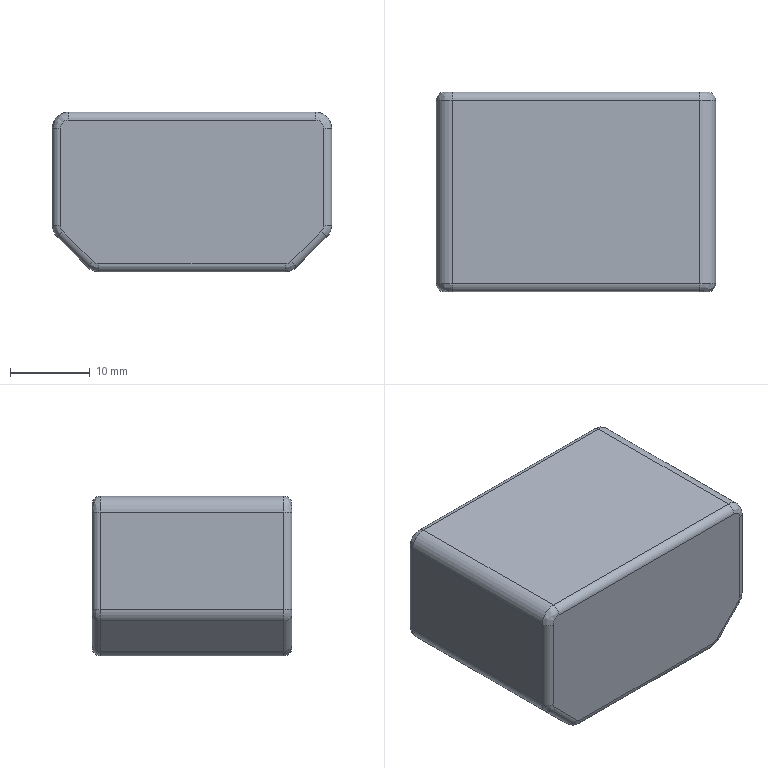Part | STEP file | 车灯-后视镜_id378_x_t | 1 solid | 38 faces | box 35 x 25 x 20 mm | volume 16780 mm3 | cylinder 18 | spline 12 | plane 8 | commonest cylinder face diameters 2 x12 4 x6
STEP:
#1=CARTESIAN_POINT('',(68.,-286.,-247.5));
#2=VERTEX_POINT('',#1);
#3=CARTESIAN_POINT('',(68.,-309.,-247.5));
#4=VERTEX_POINT('',#3);
#5=CARTESIAN_POINT('',(68.,-300.,-247.5));
#6=DIRECTION('',(0.,-1.,0.));
#7=VECTOR('',#6,1.);
#8=LINE('',#5,#7);
#9=EDGE_CURVE('',#2,#4,#8,.T.);
#10=ORIENTED_EDGE('',*,*,#9,.T.);
#11=CARTESIAN_POINT('',(99.,-309.,-247.5));
#12=VERTEX_POINT('',#11);
#13=CARTESIAN_POINT('',(83.5,-309.,-247.5));
#14=DIRECTION('',(1.,0.,0.));
#15=VECTOR('',#14,1.);
#16=LINE('',#13,#15);
#17=EDGE_CURVE('',#4,#12,#16,.T.);
#18=ORIENTED_EDGE('',*,*,#17,.T.);
#19=CARTESIAN_POINT('',(99.,-286.,-247.5));
#20=VERTEX_POINT('',#19);
#21=CARTESIAN_POINT('',(99.,-300.,-247.5));
#22=DIRECTION('',(0.,1.,0.));
#23=VECTOR('',#22,1.);
#24=LINE('',#21,#23);
#25=EDGE_CURVE('',#12,#20,#24,.T.);
#26=ORIENTED_EDGE('',*,*,#25,.T.);
#27=CARTESIAN_POINT('',(83.5,-286.,-247.5));
#28=DIRECTION('',(-1.,0.,0.));
#29=VECTOR('',#28,1.);
#30=LINE('',#27,#29);
#31=EDGE_CURVE('',#20,#2,#30,.T.);
#32=ORIENTED_EDGE('',*,*,#31,.T.);
#33=EDGE_LOOP('',(#10,#18,#26,#32));
#34=FACE_OUTER_BOUND('',#33,.T.);
#35=CARTESIAN_POINT('',(83.5,-300.,-247.5));
#36=DIRECTION('',(0.,0.,1.));
#37=DIRECTION('',(1.,0.,0.));
#38=AXIS2_PLACEMENT_3D('',#35,#36,#37);
#39=PLANE('',#38);
#40=ADVANCED_FACE('',(#34),#39,.T.);
#41=CARTESIAN_POINT('',(100.,-310.,-261.672));
#42=VERTEX_POINT('',#41);
#43=CARTESIAN_POINT('',(100.,-310.,-249.5));
#44=VERTEX_POINT('',#43);
#45=CARTESIAN_POINT('',(100.,-310.,-267.5));
#46=DIRECTION('',(0.,0.,1.));
#47=VECTOR('',#46,1.);
#48=LINE('',#45,#47);
#49=EDGE_CURVE('',#42,#44,#48,.T.);
#50=ORIENTED_EDGE('',*,*,#49,.T.);
#51=CARTESIAN_POINT('',(99.,-310.,-248.5));
#52=VERTEX_POINT('',#51);
#53=CARTESIAN_POINT('',(99.,-310.,-249.5));
#54=DIRECTION('',(0.,-1.,0.));
#55=DIRECTION('',(0.,0.,-1.));
#56=AXIS2_PLACEMENT_3D('',#53,#54,#55);
#57=CIRCLE('',#56,1.);
#58=EDGE_CURVE('',#44,#52,#57,.T.);
#59=ORIENTED_EDGE('',*,*,#58,.T.);
#60=CARTESIAN_POINT('',(68.,-310.,-248.5));
#61=VERTEX_POINT('',#60);
#62=CARTESIAN_POINT('',(83.5,-310.,-248.5));
#63=DIRECTION('',(-1.,0.,0.));
#64=VECTOR('',#63,1.);
#65=LINE('',#62,#64);
#66=EDGE_CURVE('',#52,#61,#65,.T.);
#67=ORIENTED_EDGE('',*,*,#66,.T.);
#68=CARTESIAN_POINT('',(67.,-310.,-249.5));
#69=VERTEX_POINT('',#68);
#70=CARTESIAN_POINT('',(68.,-310.,-249.5));
#71=DIRECTION('',(0.,-1.,0.));
#72=DIRECTION('',(0.,0.,-1.));
#73=AXIS2_PLACEMENT_3D('',#70,#71,#72);
#74=CIRCLE('',#73,1.);
#75=EDGE_CURVE('',#61,#69,#74,.T.);
#76=ORIENTED_EDGE('',*,*,#75,.T.);
#77=CARTESIAN_POINT('',(67.,-310.,-261.672));
#78=VERTEX_POINT('',#77);
#79=CARTESIAN_POINT('',(67.,-310.,-267.5));
#80=DIRECTION('',(0.,0.,-1.));
#81=VECTOR('',#80,1.);
#82=LINE('',#79,#81);
#83=EDGE_CURVE('',#69,#78,#82,.T.);
#84=ORIENTED_EDGE('',*,*,#83,.T.);
#85=CARTESIAN_POINT('',(67.293,-310.,-262.379));
#86=VERTEX_POINT('',#85);
#87=CARTESIAN_POINT('',(68.,-310.,-261.672));
#88=DIRECTION('',(0.,-1.,0.));
#89=DIRECTION('',(0.,0.,-1.));
#90=AXIS2_PLACEMENT_3D('',#87,#88,#89);
#91=CIRCLE('',#90,1.);
#92=EDGE_CURVE('',#78,#86,#91,.T.);
#93=ORIENTED_EDGE('',*,*,#92,.T.);
#94=CARTESIAN_POINT('',(71.121,-310.,-266.207));
#95=VERTEX_POINT('',#94);
#96=CARTESIAN_POINT('',(77.957,-310.,-273.043));
#97=DIRECTION('',(0.7071,0.,-0.7071));
#98=VECTOR('',#97,1.);
#99=LINE('',#96,#98);
#100=EDGE_CURVE('',#86,#95,#99,.T.);
#101=ORIENTED_EDGE('',*,*,#100,.T.);
#102=CARTESIAN_POINT('',(71.828,-310.,-266.5));
#103=VERTEX_POINT('',#102);
#104=CARTESIAN_POINT('',(71.828,-310.,-265.5));
#105=DIRECTION('',(0.,-1.,0.));
#106=DIRECTION('',(0.,0.,-1.));
#107=AXIS2_PLACEMENT_3D('',#104,#105,#106);
#108=CIRCLE('',#107,1.);
#109=EDGE_CURVE('',#95,#103,#108,.T.);
#110=ORIENTED_EDGE('',*,*,#109,.T.);
#111=CARTESIAN_POINT('',(95.172,-310.,-266.5));
#112=VERTEX_POINT('',#111);
#113=CARTESIAN_POINT('',(83.5,-310.,-266.5));
#114=DIRECTION('',(1.,0.,0.));
#115=VECTOR('',#114,1.);
#116=LINE('',#113,#115);
#117=EDGE_CURVE('',#103,#112,#116,.T.);
#118=ORIENTED_EDGE('',*,*,#117,.T.);
#119=CARTESIAN_POINT('',(95.879,-310.,-266.207));
#120=VERTEX_POINT('',#119);
#121=CARTESIAN_POINT('',(95.172,-310.,-265.5));
#122=DIRECTION('',(0.,-1.,0.));
#123=DIRECTION('',(0.,0.,-1.));
#124=AXIS2_PLACEMENT_3D('',#121,#122,#123);
#125=CIRCLE('',#124,1.);
#126=EDGE_CURVE('',#112,#120,#125,.T.);
#127=ORIENTED_EDGE('',*,*,#126,.T.);
#128=CARTESIAN_POINT('',(99.707,-310.,-262.379));
#129=VERTEX_POINT('',#128);
#130=CARTESIAN_POINT('',(89.043,-310.,-273.043));
#131=DIRECTION('',(0.7071,0.,0.7071));
#132=VECTOR('',#131,1.);
#133=LINE('',#130,#132);
#134=EDGE_CURVE('',#120,#129,#133,.T.);
#135=ORIENTED_EDGE('',*,*,#134,.T.);
#136=CARTESIAN_POINT('',(99.,-310.,-261.672));
#137=DIRECTION('',(0.,-1.,0.));
#138=DIRECTION('',(0.,0.,-1.));
#139=AXIS2_PLACEMENT_3D('',#136,#137,#138);
#140=CIRCLE('',#139,1.);
#141=EDGE_CURVE('',#129,#42,#140,.T.);
#142=ORIENTED_EDGE('',*,*,#141,.T.);
#143=EDGE_LOOP('',(#50,#59,#67,#76,#84,#93,#101,#110,#118,#127,#135,#142));
#144=FACE_OUTER_BOUND('',#143,.T.);
#145=CARTESIAN_POINT('',(83.5,-310.,-267.5));
#146=DIRECTION('',(0.,-1.,0.));
#147=DIRECTION('',(0.,0.,-1.));
#148=AXIS2_PLACEMENT_3D('',#145,#146,#147);
#149=PLANE('',#148);
#150=ADVANCED_FACE('',(#144),#149,.T.);
#151=CARTESIAN_POINT('',(66.,-286.,-261.672));
#152=VERTEX_POINT('',#151);
#153=CARTESIAN_POINT('',(66.,-309.,-261.672));
#154=VERTEX_POINT('',#153);
#155=CARTESIAN_POINT('',(66.,-300.,-261.672));
#156=DIRECTION('',(0.,-1.,0.));
#157=VECTOR('',#156,1.);
#158=LINE('',#155,#157);
#159=EDGE_CURVE('',#152,#154,#158,.T.);
#160=ORIENTED_EDGE('',*,*,#159,.T.);
#161=CARTESIAN_POINT('',(66.,-309.,-249.5));
#162=VERTEX_POINT('',#161);
#163=CARTESIAN_POINT('',(66.,-309.,-267.5));
#164=DIRECTION('',(0.,0.,1.));
#165=VECTOR('',#164,1.);
#166=LINE('',#163,#165);
#167=EDGE_CURVE('',#154,#162,#166,.T.);
#168=ORIENTED_EDGE('',*,*,#167,.T.);
#169=CARTESIAN_POINT('',(66.,-286.,-249.5));
#170=VERTEX_POINT('',#169);
#171=CARTESIAN_POINT('',(66.,-300.,-249.5));
#172=DIRECTION('',(0.,1.,0.));
#173=VECTOR('',#172,1.);
#174=LINE('',#171,#173);
#175=EDGE_CURVE('',#162,#170,#174,.T.);
#176=ORIENTED_EDGE('',*,*,#175,.T.);
#177=CARTESIAN_POINT('',(66.,-286.,-267.5));
#178=DIRECTION('',(0.,0.,-1.));
#179=VECTOR('',#178,1.);
#180=LINE('',#177,#179);
#181=EDGE_CURVE('',#170,#152,#180,.T.);
#182=ORIENTED_EDGE('',*,*,#181,.T.);
#183=EDGE_LOOP('',(#160,#168,#176,#182));
#184=FACE_OUTER_BOUND('',#183,.T.);
#185=CARTESIAN_POINT('',(66.,-300.,-267.5));
#186=DIRECTION('',(-1.,0.,0.));
#187=DIRECTION('',(0.,0.,1.));
#188=AXIS2_PLACEMENT_3D('',#185,#186,#187);
#189=PLANE('',#188);
#190=ADVANCED_FACE('',(#184),#189,.T.);
#191=CARTESIAN_POINT('',(67.,-285.,-261.672));
#192=VERTEX_POINT('',#191);
#193=CARTESIAN_POINT('',(67.,-285.,-249.5));
#194=VERTEX_POINT('',#193);
#195=CARTESIAN_POINT('',(67.,-285.,-267.5));
#196=DIRECTION('',(0.,0.,1.));
#197=VECTOR('',#196,1.);
#198=LINE('',#195,#197);
#199=EDGE_CURVE('',#192,#194,#198,.T.);
#200=ORIENTED_EDGE('',*,*,#199,.T.);
#201=CARTESIAN_POINT('',(68.,-285.,-248.5));
#202=VERTEX_POINT('',#201);
#203=CARTESIAN_POINT('',(68.,-285.,-249.5));
#204=DIRECTION('',(0.,1.,0.));
#205=DIRECTION('',(0.,0.,1.));
#206=AXIS2_PLACEMENT_3D('',#203,#204,#205);
#207=CIRCLE('',#206,1.);
#208=EDGE_CURVE('',#194,#202,#207,.T.);
#209=ORIENTED_EDGE('',*,*,#208,.T.);
#210=CARTESIAN_POINT('',(99.,-285.,-248.5));
#211=VERTEX_POINT('',#210);
#212=CARTESIAN_POINT('',(83.5,-285.,-248.5));
#213=DIRECTION('',(1.,0.,0.));
#214=VECTOR('',#213,1.);
#215=LINE('',#212,#214);
#216=EDGE_CURVE('',#202,#211,#215,.T.);
#217=ORIENTED_EDGE('',*,*,#216,.T.);
#218=CARTESIAN_POINT('',(100.,-285.,-249.5));
#219=VERTEX_POINT('',#218);
#220=CARTESIAN_POINT('',(99.,-285.,-249.5));
#221=DIRECTION('',(0.,1.,0.));
#222=DIRECTION('',(0.,0.,1.));
#223=AXIS2_PLACEMENT_3D('',#220,#221,#222);
#224=CIRCLE('',#223,1.);
#225=EDGE_CURVE('',#211,#219,#224,.T.);
#226=ORIENTED_EDGE('',*,*,#225,.T.);
#227=CARTESIAN_POINT('',(100.,-285.,-261.672));
#228=VERTEX_POINT('',#227);
#229=CARTESIAN_POINT('',(100.,-285.,-267.5));
#230=DIRECTION('',(0.,0.,-1.));
#231=VECTOR('',#230,1.);
#232=LINE('',#229,#231);
#233=EDGE_CURVE('',#219,#228,#232,.T.);
#234=ORIENTED_EDGE('',*,*,#233,.T.);
#235=CARTESIAN_POINT('',(99.707,-285.,-262.379));
#236=VERTEX_POINT('',#235);
#237=CARTESIAN_POINT('',(99.,-285.,-261.672));
#238=DIRECTION('',(0.,1.,0.));
#239=DIRECTION('',(0.,0.,1.));
#240=AXIS2_PLACEMENT_3D('',#237,#238,#239);
#241=CIRCLE('',#240,1.);
#242=EDGE_CURVE('',#228,#236,#241,.T.);
#243=ORIENTED_EDGE('',*,*,#242,.T.);
#244=CARTESIAN_POINT('',(95.879,-285.,-266.207));
#245=VERTEX_POINT('',#244);
#246=CARTESIAN_POINT('',(89.043,-285.,-273.043));
#247=DIRECTION('',(-0.7071,0.,-0.7071));
#248=VECTOR('',#247,1.);
#249=LINE('',#246,#248);
#250=EDGE_CURVE('',#236,#245,#249,.T.);
#251=ORIENTED_EDGE('',*,*,#250,.T.);
#252=CARTESIAN_POINT('',(95.172,-285.,-266.5));
#253=VERTEX_POINT('',#252);
#254=CARTESIAN_POINT('',(95.172,-285.,-265.5));
#255=DIRECTION('',(0.,1.,0.));
#256=DIRECTION('',(0.,0.,1.));
#257=AXIS2_PLACEMENT_3D('',#254,#255,#256);
#258=CIRCLE('',#257,1.);
#259=EDGE_CURVE('',#245,#253,#258,.T.);
#260=ORIENTED_EDGE('',*,*,#259,.T.);
#261=CARTESIAN_POINT('',(71.828,-285.,-266.5));
#262=VERTEX_POINT('',#261);
#263=CARTESIAN_POINT('',(83.5,-285.,-266.5));
#264=DIRECTION('',(-1.,0.,0.));
#265=VECTOR('',#264,1.);
#266=LINE('',#263,#265);
#267=EDGE_CURVE('',#253,#262,#266,.T.);
#268=ORIENTED_EDGE('',*,*,#267,.T.);
#269=CARTESIAN_POINT('',(71.121,-285.,-266.207));
#270=VERTEX_POINT('',#269);
#271=CARTESIAN_POINT('',(71.828,-285.,-265.5));
#272=DIRECTION('',(0.,1.,0.));
#273=DIRECTION('',(0.,0.,1.));
#274=AXIS2_PLACEMENT_3D('',#271,#272,#273);
#275=CIRCLE('',#274,1.);
#276=EDGE_CURVE('',#262,#270,#275,.T.);
#277=ORIENTED_EDGE('',*,*,#276,.T.);
#278=CARTESIAN_POINT('',(67.293,-285.,-262.379));
#279=VERTEX_POINT('',#278);
#280=CARTESIAN_POINT('',(77.957,-285.,-273.043));
#281=DIRECTION('',(-0.7071,0.,0.7071));
#282=VECTOR('',#281,1.);
#283=LINE('',#280,#282);
#284=EDGE_CURVE('',#270,#279,#283,.T.);
#285=ORIENTED_EDGE('',*,*,#284,.T.);
#286=CARTESIAN_POINT('',(68.,-285.,-261.672));
#287=DIRECTION('',(0.,1.,0.));
#288=DIRECTION('',(0.,0.,1.));
#289=AXIS2_PLACEMENT_3D('',#286,#287,#288);
#290=CIRCLE('',#289,1.);
#291=EDGE_CURVE('',#279,#192,#290,.T.);
#292=ORIENTED_EDGE('',*,*,#291,.T.);
#293=EDGE_LOOP('',(#200,#209,#217,#226,#234,#243,#251,#260,#268,#277,#285,#292));
#294=FACE_OUTER_BOUND('',#293,.T.);
#295=CARTESIAN_POINT('',(83.5,-285.,-267.5));
#296=DIRECTION('',(0.,1.,0.));
#297=DIRECTION('',(0.,0.,1.));
#298=AXIS2_PLACEMENT_3D('',#295,#296,#297);
#299=PLANE('',#298);
#300=ADVANCED_FACE('',(#294),#299,.T.);
#301=CARTESIAN_POINT('',(95.172,-286.,-267.5));
#302=VERTEX_POINT('',#301);
#303=CARTESIAN_POINT('',(95.172,-309.,-267.5));
#304=VERTEX_POINT('',#303);
#305=CARTESIAN_POINT('',(95.172,-300.,-267.5));
#306=DIRECTION('',(0.,-1.,0.));
#307=VECTOR('',#306,1.);
#308=LINE('',#305,#307);
#309=EDGE_CURVE('',#302,#304,#308,.T.);
#310=ORIENTED_EDGE('',*,*,#309,.T.);
#311=CARTESIAN_POINT('',(71.828,-309.,-267.5));
#312=VERTEX_POINT('',#311);
#313=CARTESIAN_POINT('',(83.5,-309.,-267.5));
#314=DIRECTION('',(-1.,0.,0.));
#315=VECTOR('',#314,1.);
#316=LINE('',#313,#315);
#317=EDGE_CURVE('',#304,#312,#316,.T.);
#318=ORIENTED_EDGE('',*,*,#317,.T.);
#319=CARTESIAN_POINT('',(71.828,-286.,-267.5));
#320=VERTEX_POINT('',#319);
#321=CARTESIAN_POINT('',(71.828,-300.,-267.5));
#322=DIRECTION('',(0.,1.,0.));
#323=VECTOR('',#322,1.);
#324=LINE('',#321,#323);
#325=EDGE_CURVE('',#312,#320,#324,.T.);
#326=ORIENTED_EDGE('',*,*,#325,.T.);
#327=CARTESIAN_POINT('',(83.5,-286.,-267.5));
#328=DIRECTION('',(1.,0.,0.));
#329=VECTOR('',#328,1.);
#330=LINE('',#327,#329);
#331=EDGE_CURVE('',#320,#302,#330,.T.);
#332=ORIENTED_EDGE('',*,*,#331,.T.);
#333=EDGE_LOOP('',(#310,#318,#326,#332));
#334=FACE_OUTER_BOUND('',#333,.T.);
#335=CARTESIAN_POINT('',(83.5,-300.,-267.5));
#336=DIRECTION('',(0.,0.,-1.));
#337=DIRECTION('',(-1.,0.,0.));
#338=AXIS2_PLACEMENT_3D('',#335,#336,#337);
#339=PLANE('',#338);
#340=ADVANCED_FACE('',(#334),#339,.T.);
#341=CARTESIAN_POINT('',(101.,-286.,-249.5));
#342=VERTEX_POINT('',#341);
#343=CARTESIAN_POINT('',(101.,-309.,-249.5));
#344=VERTEX_POINT('',#343);
#345=CARTESIAN_POINT('',(101.,-300.,-249.5));
#346=DIRECTION('',(0.,-1.,0.));
#347=VECTOR('',#346,1.);
#348=LINE('',#345,#347);
#349=EDGE_CURVE('',#342,#344,#348,.T.);
#350=ORIENTED_EDGE('',*,*,#349,.T.);
#351=CARTESIAN_POINT('',(101.,-309.,-261.672));
#352=VERTEX_POINT('',#351);
#353=CARTESIAN_POINT('',(101.,-309.,-267.5));
#354=DIRECTION('',(0.,0.,-1.));
#355=VECTOR('',#354,1.);
#356=LINE('',#353,#355);
#357=EDGE_CURVE('',#344,#352,#356,.T.);
#358=ORIENTED_EDGE('',*,*,#357,.T.);
#359=CARTESIAN_POINT('',(101.,-286.,-261.672));
#360=VERTEX_POINT('',#359);
#361=CARTESIAN_POINT('',(101.,-300.,-261.672));
#362=DIRECTION('',(0.,1.,0.));
#363=VECTOR('',#362,1.);
#364=LINE('',#361,#363);
#365=EDGE_CURVE('',#352,#360,#364,.T.);
#366=ORIENTED_EDGE('',*,*,#365,.T.);
#367=CARTESIAN_POINT('',(101.,-286.,-267.5));
#368=DIRECTION('',(0.,0.,1.));
#369=VECTOR('',#368,1.);
#370=LINE('',#367,#369);
#371=EDGE_CURVE('',#360,#342,#370,.T.);
#372=ORIENTED_EDGE('',*,*,#371,.T.);
#373=EDGE_LOOP('',(#350,#358,#366,#372));
#374=FACE_OUTER_BOUND('',#373,.T.);
#375=CARTESIAN_POINT('',(101.,-300.,-267.5));
#376=DIRECTION('',(1.,0.,0.));
#377=DIRECTION('',(0.,0.,-1.));
#378=AXIS2_PLACEMENT_3D('',#375,#376,#377);
#379=PLANE('',#378);
#380=ADVANCED_FACE('',(#374),#379,.T.);
#381=CARTESIAN_POINT('',(70.414,-286.,-266.914));
#382=VERTEX_POINT('',#381);
#383=CARTESIAN_POINT('',(70.414,-309.,-266.914));
#384=VERTEX_POINT('',#383);
#385=CARTESIAN_POINT('',(70.414,-300.,-266.914));
#386=DIRECTION('',(0.,-1.,0.));
#387=VECTOR('',#386,1.);
#388=LINE('',#385,#387);
#389=EDGE_CURVE('',#382,#384,#388,.T.);
#390=ORIENTED_EDGE('',*,*,#389,.T.);
#391=CARTESIAN_POINT('',(66.586,-309.,-263.086));
#392=VERTEX_POINT('',#391);
#393=CARTESIAN_POINT('',(66.,-309.,-262.5));
#394=DIRECTION('',(-0.7071,0.,0.7071));
#395=VECTOR('',#394,1.);
#396=LINE('',#393,#395);
#397=EDGE_CURVE('',#384,#392,#396,.T.);
#398=ORIENTED_EDGE('',*,*,#397,.T.);
#399=CARTESIAN_POINT('',(66.586,-286.,-263.086));
#400=VERTEX_POINT('',#399);
#401=CARTESIAN_POINT('',(66.586,-300.,-263.086));
#402=DIRECTION('',(0.,1.,0.));
#403=VECTOR('',#402,1.);
#404=LINE('',#401,#403);
#405=EDGE_CURVE('',#392,#400,#404,.T.);
#406=ORIENTED_EDGE('',*,*,#405,.T.);
#407=CARTESIAN_POINT('',(66.,-286.,-262.5));
#408=DIRECTION('',(0.7071,0.,-0.7071));
#409=VECTOR('',#408,1.);
#410=LINE('',#407,#409);
#411=EDGE_CURVE('',#400,#382,#410,.T.);
#412=ORIENTED_EDGE('',*,*,#411,.T.);
#413=EDGE_LOOP('',(#390,#398,#406,#412));
#414=FACE_OUTER_BOUND('',#413,.T.);
#415=CARTESIAN_POINT('',(66.,-300.,-262.5));
#416=DIRECTION('',(0.7071,0.,0.7071));
#417=DIRECTION('',(0.7071,0.,-0.7071));
#418=AXIS2_PLACEMENT_3D('',#415,#416,#417);
#419=PLANE('',#418);
#420=ADVANCED_FACE('',(#414),#419,.F.);
#421=CARTESIAN_POINT('',(100.414,-286.,-263.086));
#422=VERTEX_POINT('',#421);
#423=CARTESIAN_POINT('',(100.414,-309.,-263.086));
#424=VERTEX_POINT('',#423);
#425=CARTESIAN_POINT('',(100.414,-300.,-263.086));
#426=DIRECTION('',(0.,-1.,0.));
#427=VECTOR('',#426,1.);
#428=LINE('',#425,#427);
#429=EDGE_CURVE('',#422,#424,#428,.T.);
#430=ORIENTED_EDGE('',*,*,#429,.T.);
#431=CARTESIAN_POINT('',(96.586,-309.,-266.914));
#432=VERTEX_POINT('',#431);
#433=CARTESIAN_POINT('',(101.,-309.,-262.5));
#434=DIRECTION('',(-0.7071,0.,-0.7071));
#435=VECTOR('',#434,1.);
#436=LINE('',#433,#435);
#437=EDGE_CURVE('',#424,#432,#436,.T.);
#438=ORIENTED_EDGE('',*,*,#437,.T.);
#439=CARTESIAN_POINT('',(96.586,-286.,-266.914));
#440=VERTEX_POINT('',#439);
#441=CARTESIAN_POINT('',(96.586,-300.,-266.914));
#442=DIRECTION('',(0.,1.,0.));
#443=VECTOR('',#442,1.);
#444=LINE('',#441,#443);
#445=EDGE_CURVE('',#432,#440,#444,.T.);
#446=ORIENTED_EDGE('',*,*,#445,.T.);
#447=CARTESIAN_POINT('',(101.,-286.,-262.5));
#448=DIRECTION('',(0.7071,0.,0.7071));
#449=VECTOR('',#448,1.);
#450=LINE('',#447,#449);
#451=EDGE_CURVE('',#440,#422,#450,.T.);
#452=ORIENTED_EDGE('',*,*,#451,.T.);
#453=EDGE_LOOP('',(#430,#438,#446,#452));
#454=FACE_OUTER_BOUND('',#453,.T.);
#455=CARTESIAN_POINT('',(101.,-300.,-262.5));
#456=DIRECTION('',(-0.7071,0.,0.7071));
#457=DIRECTION('',(0.7071,0.,0.7071));
#458=AXIS2_PLACEMENT_3D('',#455,#456,#457);
#459=PLANE('',#458);
#460=ADVANCED_FACE('',(#454),#459,.F.);
#461=ORIENTED_EDGE('',*,*,#445,.F.);
#462=CARTESIAN_POINT('',(95.172,-309.,-265.5));
#463=DIRECTION('',(0.,1.,0.));
#464=DIRECTION('',(0.,0.,-1.));
#465=AXIS2_PLACEMENT_3D('',#462,#463,#464);
#466=CIRCLE('',#465,2.);
#467=EDGE_CURVE('',#432,#304,#466,.T.);
#468=ORIENTED_EDGE('',*,*,#467,.T.);
#469=ORIENTED_EDGE('',*,*,#309,.F.);
#470=CARTESIAN_POINT('',(95.172,-286.,-265.5));
#471=DIRECTION('',(0.,-1.,0.));
#472=DIRECTION('',(0.,0.,1.));
#473=AXIS2_PLACEMENT_3D('',#470,#471,#472);
#474=CIRCLE('',#473,2.);
#475=EDGE_CURVE('',#302,#440,#474,.T.);
#476=ORIENTED_EDGE('',*,*,#475,.T.);
#477=EDGE_LOOP('',(#461,#468,#469,#476));
#478=FACE_OUTER_BOUND('',#477,.T.);
#479=CARTESIAN_POINT('',(95.172,-300.,-265.5));
#480=DIRECTION('',(0.,1.,0.));
#481=DIRECTION('',(0.,0.,1.));
#482=AXIS2_PLACEMENT_3D('',#479,#480,#481);
#483=CYLINDRICAL_SURFACE('',#482,2.);
#484=ADVANCED_FACE('',(#478),#483,.T.);
#485=ORIENTED_EDGE('',*,*,#365,.F.);
#486=CARTESIAN_POINT('',(99.,-309.,-261.672));
#487=DIRECTION('',(0.,1.,0.));
#488=DIRECTION('',(0.,0.,-1.));
#489=AXIS2_PLACEMENT_3D('',#486,#487,#488);
#490=CIRCLE('',#489,2.);
#491=EDGE_CURVE('',#352,#424,#490,.T.);
#492=ORIENTED_EDGE('',*,*,#491,.T.);
#493=ORIENTED_EDGE('',*,*,#429,.F.);
#494=CARTESIAN_POINT('',(99.,-286.,-261.672));
#495=DIRECTION('',(0.,-1.,0.));
#496=DIRECTION('',(0.,0.,1.));
#497=AXIS2_PLACEMENT_3D('',#494,#495,#496);
#498=CIRCLE('',#497,2.);
#499=EDGE_CURVE('',#422,#360,#498,.T.);
#500=ORIENTED_EDGE('',*,*,#499,.T.);
#501=EDGE_LOOP('',(#485,#492,#493,#500));
#502=FACE_OUTER_BOUND('',#501,.T.);
#503=CARTESIAN_POINT('',(99.,-300.,-261.672));
#504=DIRECTION('',(0.,-1.,0.));
#505=DIRECTION('',(0.,0.,-1.));
#506=AXIS2_PLACEMENT_3D('',#503,#504,#505);
#507=CYLINDRICAL_SURFACE('',#506,2.);
#508=ADVANCED_FACE('',(#502),#507,.T.);
#509=ORIENTED_EDGE('',*,*,#25,.F.);
#510=CARTESIAN_POINT('',(99.,-309.,-249.5));
#511=DIRECTION('',(0.,1.,0.));
#512=DIRECTION('',(0.,0.,-1.));
#513=AXIS2_PLACEMENT_3D('',#510,#511,#512);
#514=CIRCLE('',#513,2.);
#515=EDGE_CURVE('',#12,#344,#514,.T.);
#516=ORIENTED_EDGE('',*,*,#515,.T.);
#517=ORIENTED_EDGE('',*,*,#349,.F.);
#518=CARTESIAN_POINT('',(99.,-286.,-249.5));
#519=DIRECTION('',(0.,-1.,0.));
#520=DIRECTION('',(0.,0.,1.));
#521=AXIS2_PLACEMENT_3D('',#518,#519,#520);
#522=CIRCLE('',#521,2.);
#523=EDGE_CURVE('',#342,#20,#522,.T.);
#524=ORIENTED_EDGE('',*,*,#523,.T.);
#525=EDGE_LOOP('',(#509,#516,#517,#524));
#526=FACE_OUTER_BOUND('',#525,.T.);
#527=CARTESIAN_POINT('',(99.,-300.,-249.5));
#528=DIRECTION('',(0.,-1.,0.));
#529=DIRECTION('',(0.,0.,-1.));
#530=AXIS2_PLACEMENT_3D('',#527,#528,#529);
#531=CYLINDRICAL_SURFACE('',#530,2.);
#532=ADVANCED_FACE('',(#526),#531,.T.);
#533=ORIENTED_EDGE('',*,*,#175,.F.);
#534=CARTESIAN_POINT('',(68.,-309.,-249.5));
#535=DIRECTION('',(0.,1.,0.));
#536=DIRECTION('',(0.,0.,-1.));
#537=AXIS2_PLACEMENT_3D('',#534,#535,#536);
#538=CIRCLE('',#537,2.);
#539=EDGE_CURVE('',#162,#4,#538,.T.);
#540=ORIENTED_EDGE('',*,*,#539,.T.);
#541=ORIENTED_EDGE('',*,*,#9,.F.);
#542=CARTESIAN_POINT('',(68.,-286.,-249.5));
#543=DIRECTION('',(0.,-1.,0.));
#544=DIRECTION('',(0.,0.,1.));
#545=AXIS2_PLACEMENT_3D('',#542,#543,#544);
#546=CIRCLE('',#545,2.);
#547=EDGE_CURVE('',#2,#170,#546,.T.);
#548=ORIENTED_EDGE('',*,*,#547,.T.);
#549=EDGE_LOOP('',(#533,#540,#541,#548));
#550=FACE_OUTER_BOUND('',#549,.T.);
#551=CARTESIAN_POINT('',(68.,-300.,-249.5));
#552=DIRECTION('',(0.,1.,0.));
#553=DIRECTION('',(0.,0.,1.));
#554=AXIS2_PLACEMENT_3D('',#551,#552,#553);
#555=CYLINDRICAL_SURFACE('',#554,2.);
#556=ADVANCED_FACE('',(#550),#555,.T.);
#557=ORIENTED_EDGE('',*,*,#325,.F.);
#558=CARTESIAN_POINT('',(71.828,-309.,-265.5));
#559=DIRECTION('',(0.,1.,0.));
#560=DIRECTION('',(0.,0.,-1.));
#561=AXIS2_PLACEMENT_3D('',#558,#559,#560);
#562=CIRCLE('',#561,2.);
#563=EDGE_CURVE('',#312,#384,#562,.T.);
#564=ORIENTED_EDGE('',*,*,#563,.T.);
#565=ORIENTED_EDGE('',*,*,#389,.F.);
#566=CARTESIAN_POINT('',(71.828,-286.,-265.5));
#567=DIRECTION('',(0.,-1.,0.));
#568=DIRECTION('',(0.,0.,1.));
#569=AXIS2_PLACEMENT_3D('',#566,#567,#568);
#570=CIRCLE('',#569,2.);
#571=EDGE_CURVE('',#382,#320,#570,.T.);
#572=ORIENTED_EDGE('',*,*,#571,.T.);
#573=EDGE_LOOP('',(#557,#564,#565,#572));
#574=FACE_OUTER_BOUND('',#573,.T.);
#575=CARTESIAN_POINT('',(71.828,-300.,-265.5));
#576=DIRECTION('',(0.,-1.,0.));
#577=DIRECTION('',(0.,0.,-1.));
#578=AXIS2_PLACEMENT_3D('',#575,#576,#577);
#579=CYLINDRICAL_SURFACE('',#578,2.);
#580=ADVANCED_FACE('',(#574),#579,.T.);
#581=ORIENTED_EDGE('',*,*,#405,.F.);
#582=CARTESIAN_POINT('',(68.,-309.,-261.672));
#583=DIRECTION('',(0.,1.,0.));
#584=DIRECTION('',(0.,0.,-1.));
#585=AXIS2_PLACEMENT_3D('',#582,#583,#584);
#586=CIRCLE('',#585,2.);
#587=EDGE_CURVE('',#392,#154,#586,.T.);
#588=ORIENTED_EDGE('',*,*,#587,.T.);
#589=ORIENTED_EDGE('',*,*,#159,.F.);
#590=CARTESIAN_POINT('',(68.,-286.,-261.672));
#591=DIRECTION('',(0.,-1.,0.));
#592=DIRECTION('',(0.,0.,1.));
#593=AXIS2_PLACEMENT_3D('',#590,#591,#592);
#594=CIRCLE('',#593,2.);
#595=EDGE_CURVE('',#152,#400,#594,.T.);
#596=ORIENTED_EDGE('',*,*,#595,.T.);
#597=EDGE_LOOP('',(#581,#588,#589,#596));
#598=FACE_OUTER_BOUND('',#597,.T.);
#599=CARTESIAN_POINT('',(68.,-300.,-261.672));
#600=DIRECTION('',(0.,1.,0.));
#601=DIRECTION('',(0.,0.,1.));
#602=AXIS2_PLACEMENT_3D('',#599,#600,#601);
#603=CYLINDRICAL_SURFACE('',#602,2.);
#604=ADVANCED_FACE('',(#598),#603,.T.);
#605=CARTESIAN_POINT('',(71.121,-309.,-266.207));
#606=DIRECTION('',(-0.7071,0.,0.7071));
#607=DIRECTION('',(0.7071,0.,0.7071));
#608=AXIS2_PLACEMENT_3D('',#605,#606,#607);
#609=CIRCLE('',#608,1.);
#610=EDGE_CURVE('',#384,#95,#609,.T.);
#611=ORIENTED_EDGE('',*,*,#610,.F.);
#612=ORIENTED_EDGE('',*,*,#563,.F.);
#613=CARTESIAN_POINT('',(71.828,-309.,-266.5));
#614=DIRECTION('',(1.,0.,0.));
#615=DIRECTION('',(0.,0.,-1.));
#616=AXIS2_PLACEMENT_3D('',#613,#614,#615);
#617=CIRCLE('',#616,1.);
#618=EDGE_CURVE('',#103,#312,#617,.T.);
#619=ORIENTED_EDGE('',*,*,#618,.F.);
#620=ORIENTED_EDGE('',*,*,#109,.F.);
#621=EDGE_LOOP('',(#611,#612,#619,#620));
#622=FACE_OUTER_BOUND('',#621,.T.);
#623=CARTESIAN_POINT('',(71.121,-310.,-266.207));
#624=CARTESIAN_POINT('',(71.311,-310.,-266.397));
#625=CARTESIAN_POINT('',(71.56,-310.,-266.5));
#626=CARTESIAN_POINT('',(71.828,-310.,-266.5));
#627=CARTESIAN_POINT('',(70.707,-310.,-266.621));
#628=CARTESIAN_POINT('',(71.008,-310.,-266.923));
#629=CARTESIAN_POINT('',(71.402,-310.,-267.086));
#630=CARTESIAN_POINT('',(71.828,-310.,-267.086));
#631=CARTESIAN_POINT('',(70.414,-309.586,-266.914));
#632=CARTESIAN_POINT('',(70.794,-309.586,-267.294));
#633=CARTESIAN_POINT('',(71.291,-309.586,-267.5));
#634=CARTESIAN_POINT('',(71.828,-309.586,-267.5));
#635=CARTESIAN_POINT('',(70.414,-309.,-266.914));
#636=CARTESIAN_POINT('',(70.794,-309.,-267.294));
#637=CARTESIAN_POINT('',(71.291,-309.,-267.5));
#638=CARTESIAN_POINT('',(71.828,-309.,-267.5));
#639=(BOUNDED_SURFACE()B_SPLINE_SURFACE(3,3,((#623,#624,#625,#626),(#627,#628,#629,#630),(#631,#632,#633,#634),(#635,#636,#637,#638)),.UNSPECIFIED.,.F.,.F.,.F.)B_SPLINE_SURFACE_WITH_KNOTS((4,4),(4,4),(0.,1.),(0.,1.),.UNSPECIFIED.)GEOMETRIC_REPRESENTATION_ITEM()RATIONAL_B_SPLINE_SURFACE(((1.,0.9493,0.9493,1.),(0.8047,0.7639,0.7639,0.8047),(0.8047,0.7639,0.7639,0.8047),(1.,0.9493,0.9493,1.)))REPRESENTATION_ITEM('')SURFACE());
#640=ADVANCED_FACE('',(#622),#639,.T.);
#641=ORIENTED_EDGE('',*,*,#618,.T.);
#642=ORIENTED_EDGE('',*,*,#317,.F.);
#643=CARTESIAN_POINT('',(95.172,-309.,-266.5));
#644=DIRECTION('',(1.,0.,0.));
#645=DIRECTION('',(0.,0.,-1.));
#646=AXIS2_PLACEMENT_3D('',#643,#644,#645);
#647=CIRCLE('',#646,1.);
#648=EDGE_CURVE('',#112,#304,#647,.T.);
#649=ORIENTED_EDGE('',*,*,#648,.F.);
#650=ORIENTED_EDGE('',*,*,#117,.F.);
#651=EDGE_LOOP('',(#641,#642,#649,#650));
#652=FACE_OUTER_BOUND('',#651,.T.);
#653=CARTESIAN_POINT('',(83.5,-309.,-266.5));
#654=DIRECTION('',(1.,0.,0.));
#655=DIRECTION('',(0.,0.,-1.));
#656=AXIS2_PLACEMENT_3D('',#653,#654,#655);
#657=CYLINDRICAL_SURFACE('',#656,1.);
#658=ADVANCED_FACE('',(#652),#657,.T.);
#659=ORIENTED_EDGE('',*,*,#610,.T.);
#660=ORIENTED_EDGE('',*,*,#100,.F.);
#661=CARTESIAN_POINT('',(67.293,-309.,-262.379));
#662=DIRECTION('',(-0.7071,0.,0.7071));
#663=DIRECTION('',(0.7071,0.,0.7071));
#664=AXIS2_PLACEMENT_3D('',#661,#662,#663);
#665=CIRCLE('',#664,1.);
#666=EDGE_CURVE('',#392,#86,#665,.T.);
#667=ORIENTED_EDGE('',*,*,#666,.F.);
#668=ORIENTED_EDGE('',*,*,#397,.F.);
#669=EDGE_LOOP('',(#659,#660,#667,#668));
#670=FACE_OUTER_BOUND('',#669,.T.);
#671=CARTESIAN_POINT('',(77.957,-309.,-273.043));
#672=DIRECTION('',(-0.7071,0.,0.7071));
#673=DIRECTION('',(0.7071,0.,0.7071));
#674=AXIS2_PLACEMENT_3D('',#671,#672,#673);
#675=CYLINDRICAL_SURFACE('',#674,1.);
#676=ADVANCED_FACE('',(#670),#675,.T.);
#677=ORIENTED_EDGE('',*,*,#648,.T.);
#678=ORIENTED_EDGE('',*,*,#467,.F.);
#679=CARTESIAN_POINT('',(95.879,-309.,-266.207));
#680=DIRECTION('',(0.7071,0.,0.7071));
#681=DIRECTION('',(0.7071,0.,-0.7071));
#682=AXIS2_PLACEMENT_3D('',#679,#680,#681);
#683=CIRCLE('',#682,1.);
#684=EDGE_CURVE('',#120,#432,#683,.T.);
#685=ORIENTED_EDGE('',*,*,#684,.F.);
#686=ORIENTED_EDGE('',*,*,#126,.F.);
#687=EDGE_LOOP('',(#677,#678,#685,#686));
#688=FACE_OUTER_BOUND('',#687,.T.);
#689=CARTESIAN_POINT('',(95.172,-310.,-266.5));
#690=CARTESIAN_POINT('',(95.44,-310.,-266.5));
#691=CARTESIAN_POINT('',(95.689,-310.,-266.397));
#692=CARTESIAN_POINT('',(95.879,-310.,-266.207));
#693=CARTESIAN_POINT('',(95.172,-310.,-267.086));
#694=CARTESIAN_POINT('',(95.598,-310.,-267.086));
#695=CARTESIAN_POINT('',(95.992,-310.,-266.923));
#696=CARTESIAN_POINT('',(96.293,-310.,-266.621));
#697=CARTESIAN_POINT('',(95.172,-309.586,-267.5));
#698=CARTESIAN_POINT('',(95.709,-309.586,-267.5));
#699=CARTESIAN_POINT('',(96.206,-309.586,-267.294));
#700=CARTESIAN_POINT('',(96.586,-309.586,-266.914));
#701=CARTESIAN_POINT('',(95.172,-309.,-267.5));
#702=CARTESIAN_POINT('',(95.709,-309.,-267.5));
#703=CARTESIAN_POINT('',(96.206,-309.,-267.294));
#704=CARTESIAN_POINT('',(96.586,-309.,-266.914));
#705=(BOUNDED_SURFACE()B_SPLINE_SURFACE(3,3,((#689,#690,#691,#692),(#693,#694,#695,#696),(#697,#698,#699,#700),(#701,#702,#703,#704)),.UNSPECIFIED.,.F.,.F.,.F.)B_SPLINE_SURFACE_WITH_KNOTS((4,4),(4,4),(0.,1.),(0.,1.),.UNSPECIFIED.)GEOMETRIC_REPRESENTATION_ITEM()RATIONAL_B_SPLINE_SURFACE(((1.,0.9493,0.9493,1.),(0.8047,0.7639,0.7639,0.8047),(0.8047,0.7639,0.7639,0.8047),(1.,0.9493,0.9493,1.)))REPRESENTATION_ITEM('')SURFACE());
#706=ADVANCED_FACE('',(#688),#705,.T.);
#707=ORIENTED_EDGE('',*,*,#666,.T.);
#708=ORIENTED_EDGE('',*,*,#92,.F.);
#709=CARTESIAN_POINT('',(67.,-309.,-261.672));
#710=DIRECTION('',(0.,0.,1.));
#711=DIRECTION('',(1.,0.,0.));
#712=AXIS2_PLACEMENT_3D('',#709,#710,#711);
#713=CIRCLE('',#712,1.);
#714=EDGE_CURVE('',#154,#78,#713,.T.);
#715=ORIENTED_EDGE('',*,*,#714,.F.);
#716=ORIENTED_EDGE('',*,*,#587,.F.);
#717=EDGE_LOOP('',(#707,#708,#715,#716));
#718=FACE_OUTER_BOUND('',#717,.T.);
#719=CARTESIAN_POINT('',(67.,-310.,-261.672));
#720=CARTESIAN_POINT('',(67.,-310.,-261.94));
#721=CARTESIAN_POINT('',(67.103,-310.,-262.189));
#722=CARTESIAN_POINT('',(67.293,-310.,-262.379));
#723=CARTESIAN_POINT('',(66.414,-310.,-261.672));
#724=CARTESIAN_POINT('',(66.414,-310.,-262.098));
#725=CARTESIAN_POINT('',(66.577,-310.,-262.492));
#726=CARTESIAN_POINT('',(66.879,-310.,-262.793));
#727=CARTESIAN_POINT('',(66.,-309.586,-261.672));
#728=CARTESIAN_POINT('',(66.,-309.586,-262.209));
#729=CARTESIAN_POINT('',(66.206,-309.586,-262.706));
#730=CARTESIAN_POINT('',(66.586,-309.586,-263.086));
#731=CARTESIAN_POINT('',(66.,-309.,-261.672));
#732=CARTESIAN_POINT('',(66.,-309.,-262.209));
#733=CARTESIAN_POINT('',(66.206,-309.,-262.706));
#734=CARTESIAN_POINT('',(66.586,-309.,-263.086));
#735=(BOUNDED_SURFACE()B_SPLINE_SURFACE(3,3,((#719,#720,#721,#722),(#723,#724,#725,#726),(#727,#728,#729,#730),(#731,#732,#733,#734)),.UNSPECIFIED.,.F.,.F.,.F.)B_SPLINE_SURFACE_WITH_KNOTS((4,4),(4,4),(0.,1.),(0.,1.),.UNSPECIFIED.)GEOMETRIC_REPRESENTATION_ITEM()RATIONAL_B_SPLINE_SURFACE(((1.,0.9493,0.9493,1.),(0.8047,0.7639,0.7639,0.8047),(0.8047,0.7639,0.7639,0.8047),(1.,0.9493,0.9493,1.)))REPRESENTATION_ITEM('')SURFACE());
#736=ADVANCED_FACE('',(#718),#735,.T.);
#737=ORIENTED_EDGE('',*,*,#684,.T.);
#738=ORIENTED_EDGE('',*,*,#437,.F.);
#739=CARTESIAN_POINT('',(99.707,-309.,-262.379));
#740=DIRECTION('',(0.7071,0.,0.7071));
#741=DIRECTION('',(0.7071,0.,-0.7071));
#742=AXIS2_PLACEMENT_3D('',#739,#740,#741);
#743=CIRCLE('',#742,1.);
#744=EDGE_CURVE('',#129,#424,#743,.T.);
#745=ORIENTED_EDGE('',*,*,#744,.F.);
#746=ORIENTED_EDGE('',*,*,#134,.F.);
#747=EDGE_LOOP('',(#737,#738,#745,#746));
#748=FACE_OUTER_BOUND('',#747,.T.);
#749=CARTESIAN_POINT('',(89.043,-309.,-273.043));
#750=DIRECTION('',(-0.7071,0.,-0.7071));
#751=DIRECTION('',(-0.7071,0.,0.7071));
#752=AXIS2_PLACEMENT_3D('',#749,#750,#751);
#753=CYLINDRICAL_SURFACE('',#752,1.);
#754=ADVANCED_FACE('',(#748),#753,.T.);
#755=ORIENTED_EDGE('',*,*,#714,.T.);
#756=ORIENTED_EDGE('',*,*,#83,.F.);
#757=CARTESIAN_POINT('',(67.,-309.,-249.5));
#758=DIRECTION('',(0.,0.,1.));
#759=DIRECTION('',(1.,0.,0.));
#760=AXIS2_PLACEMENT_3D('',#757,#758,#759);
#761=CIRCLE('',#760,1.);
#762=EDGE_CURVE('',#162,#69,#761,.T.);
#763=ORIENTED_EDGE('',*,*,#762,.F.);
#764=ORIENTED_EDGE('',*,*,#167,.F.);
#765=EDGE_LOOP('',(#755,#756,#763,#764));
#766=FACE_OUTER_BOUND('',#765,.T.);
#767=CARTESIAN_POINT('',(67.,-309.,-267.5));
#768=DIRECTION('',(0.,0.,1.));
#769=DIRECTION('',(1.,0.,0.));
#770=AXIS2_PLACEMENT_3D('',#767,#768,#769);
#771=CYLINDRICAL_SURFACE('',#770,1.);
#772=ADVANCED_FACE('',(#766),#771,.T.);
#773=ORIENTED_EDGE('',*,*,#744,.T.);
#774=ORIENTED_EDGE('',*,*,#491,.F.);
#775=CARTESIAN_POINT('',(100.,-309.,-261.672));
#776=DIRECTION('',(0.,0.,1.));
#777=DIRECTION('',(1.,0.,0.));
#778=AXIS2_PLACEMENT_3D('',#775,#776,#777);
#779=CIRCLE('',#778,1.);
#780=EDGE_CURVE('',#42,#352,#779,.T.);
#781=ORIENTED_EDGE('',*,*,#780,.F.);
#782=ORIENTED_EDGE('',*,*,#141,.F.);
#783=EDGE_LOOP('',(#773,#774,#781,#782));
#784=FACE_OUTER_BOUND('',#783,.T.);
#785=CARTESIAN_POINT('',(99.707,-310.,-262.379));
#786=CARTESIAN_POINT('',(99.897,-310.,-262.189));
#787=CARTESIAN_POINT('',(100.,-310.,-261.94));
#788=CARTESIAN_POINT('',(100.,-310.,-261.672));
#789=CARTESIAN_POINT('',(100.121,-310.,-262.793));
#790=CARTESIAN_POINT('',(100.423,-310.,-262.492));
#791=CARTESIAN_POINT('',(100.586,-310.,-262.098));
#792=CARTESIAN_POINT('',(100.586,-310.,-261.672));
#793=CARTESIAN_POINT('',(100.414,-309.586,-263.086));
#794=CARTESIAN_POINT('',(100.794,-309.586,-262.706));
#795=CARTESIAN_POINT('',(101.,-309.586,-262.209));
#796=CARTESIAN_POINT('',(101.,-309.586,-261.672));
#797=CARTESIAN_POINT('',(100.414,-309.,-263.086));
#798=CARTESIAN_POINT('',(100.794,-309.,-262.706));
#799=CARTESIAN_POINT('',(101.,-309.,-262.209));
#800=CARTESIAN_POINT('',(101.,-309.,-261.672));
#801=(BOUNDED_SURFACE()B_SPLINE_SURFACE(3,3,((#785,#786,#787,#788),(#789,#790,#791,#792),(#793,#794,#795,#796),(#797,#798,#799,#800)),.UNSPECIFIED.,.F.,.F.,.F.)B_SPLINE_SURFACE_WITH_KNOTS((4,4),(4,4),(0.,1.),(0.,1.),.UNSPECIFIED.)GEOMETRIC_REPRESENTATION_ITEM()RATIONAL_B_SPLINE_SURFACE(((1.,0.9493,0.9493,1.),(0.8047,0.7639,0.7639,0.8047),(0.8047,0.7639,0.7639,0.8047),(1.,0.9493,0.9493,1.)))REPRESENTATION_ITEM('')SURFACE());
#802=ADVANCED_FACE('',(#784),#801,.T.);
#803=ORIENTED_EDGE('',*,*,#762,.T.);
#804=ORIENTED_EDGE('',*,*,#75,.F.);
#805=CARTESIAN_POINT('',(68.,-309.,-248.5));
#806=DIRECTION('',(1.,0.,0.));
#807=DIRECTION('',(0.,0.,-1.));
#808=AXIS2_PLACEMENT_3D('',#805,#806,#807);
#809=CIRCLE('',#808,1.);
#810=EDGE_CURVE('',#4,#61,#809,.T.);
#811=ORIENTED_EDGE('',*,*,#810,.F.);
#812=ORIENTED_EDGE('',*,*,#539,.F.);
#813=EDGE_LOOP('',(#803,#804,#811,#812));
#814=FACE_OUTER_BOUND('',#813,.T.);
#815=CARTESIAN_POINT('',(68.,-310.,-248.5));
#816=CARTESIAN_POINT('',(67.414,-310.,-248.5));
#817=CARTESIAN_POINT('',(67.,-310.,-248.914));
#818=CARTESIAN_POINT('',(67.,-310.,-249.5));
#819=CARTESIAN_POINT('',(68.,-310.,-247.914));
#820=CARTESIAN_POINT('',(67.071,-310.,-247.914));
#821=CARTESIAN_POINT('',(66.414,-310.,-248.571));
#822=CARTESIAN_POINT('',(66.414,-310.,-249.5));
#823=CARTESIAN_POINT('',(68.,-309.586,-247.5));
#824=CARTESIAN_POINT('',(66.828,-309.586,-247.5));
#825=CARTESIAN_POINT('',(66.,-309.586,-248.328));
#826=CARTESIAN_POINT('',(66.,-309.586,-249.5));
#827=CARTESIAN_POINT('',(68.,-309.,-247.5));
#828=CARTESIAN_POINT('',(66.828,-309.,-247.5));
#829=CARTESIAN_POINT('',(66.,-309.,-248.328));
#830=CARTESIAN_POINT('',(66.,-309.,-249.5));
#831=(BOUNDED_SURFACE()B_SPLINE_SURFACE(3,3,((#815,#816,#817,#818),(#819,#820,#821,#822),(#823,#824,#825,#826),(#827,#828,#829,#830)),.UNSPECIFIED.,.F.,.F.,.F.)B_SPLINE_SURFACE_WITH_KNOTS((4,4),(4,4),(0.,1.),(0.,1.),.UNSPECIFIED.)GEOMETRIC_REPRESENTATION_ITEM()RATIONAL_B_SPLINE_SURFACE(((1.,0.8047,0.8047,1.),(0.8047,0.6476,0.6476,0.8047),(0.8047,0.6476,0.6476,0.8047),(1.,0.8047,0.8047,1.)))REPRESENTATION_ITEM('')SURFACE());
#832=ADVANCED_FACE('',(#814),#831,.T.);
#833=ORIENTED_EDGE('',*,*,#780,.T.);
#834=ORIENTED_EDGE('',*,*,#357,.F.);
#835=CARTESIAN_POINT('',(100.,-309.,-249.5));
#836=DIRECTION('',(0.,0.,1.));
#837=DIRECTION('',(1.,0.,0.));
#838=AXIS2_PLACEMENT_3D('',#835,#836,#837);
#839=CIRCLE('',#838,1.);
#840=EDGE_CURVE('',#44,#344,#839,.T.);
#841=ORIENTED_EDGE('',*,*,#840,.F.);
#842=ORIENTED_EDGE('',*,*,#49,.F.);
#843=EDGE_LOOP('',(#833,#834,#841,#842));
#844=FACE_OUTER_BOUND('',#843,.T.);
#845=CARTESIAN_POINT('',(100.,-309.,-267.5));
#846=DIRECTION('',(0.,0.,1.));
#847=DIRECTION('',(1.,0.,0.));
#848=AXIS2_PLACEMENT_3D('',#845,#846,#847);
#849=CYLINDRICAL_SURFACE('',#848,1.);
#850=ADVANCED_FACE('',(#844),#849,.T.);
#851=ORIENTED_EDGE('',*,*,#810,.T.);
#852=ORIENTED_EDGE('',*,*,#66,.F.);
#853=CARTESIAN_POINT('',(99.,-309.,-248.5));
#854=DIRECTION('',(1.,0.,0.));
#855=DIRECTION('',(0.,0.,-1.));
#856=AXIS2_PLACEMENT_3D('',#853,#854,#855);
#857=CIRCLE('',#856,1.);
#858=EDGE_CURVE('',#12,#52,#857,.T.);
#859=ORIENTED_EDGE('',*,*,#858,.F.);
#860=ORIENTED_EDGE('',*,*,#17,.F.);
#861=EDGE_LOOP('',(#851,#852,#859,#860));
#862=FACE_OUTER_BOUND('',#861,.T.);
#863=CARTESIAN_POINT('',(83.5,-309.,-248.5));
#864=DIRECTION('',(-1.,0.,0.));
#865=DIRECTION('',(0.,0.,1.));
#866=AXIS2_PLACEMENT_3D('',#863,#864,#865);
#867=CYLINDRICAL_SURFACE('',#866,1.);
#868=ADVANCED_FACE('',(#862),#867,.T.);
#869=ORIENTED_EDGE('',*,*,#840,.T.);
#870=ORIENTED_EDGE('',*,*,#515,.F.);
#871=ORIENTED_EDGE('',*,*,#858,.T.);
#872=ORIENTED_EDGE('',*,*,#58,.F.);
#873=EDGE_LOOP('',(#869,#870,#871,#872));
#874=FACE_OUTER_BOUND('',#873,.T.);
#875=CARTESIAN_POINT('',(100.,-310.,-249.5));
#876=CARTESIAN_POINT('',(100.,-310.,-248.914));
#877=CARTESIAN_POINT('',(99.586,-310.,-248.5));
#878=CARTESIAN_POINT('',(99.,-310.,-248.5));
#879=CARTESIAN_POINT('',(100.586,-310.,-249.5));
#880=CARTESIAN_POINT('',(100.586,-310.,-248.571));
#881=CARTESIAN_POINT('',(99.929,-310.,-247.914));
#882=CARTESIAN_POINT('',(99.,-310.,-247.914));
#883=CARTESIAN_POINT('',(101.,-309.586,-249.5));
#884=CARTESIAN_POINT('',(101.,-309.586,-248.328));
#885=CARTESIAN_POINT('',(100.172,-309.586,-247.5));
#886=CARTESIAN_POINT('',(99.,-309.586,-247.5));
#887=CARTESIAN_POINT('',(101.,-309.,-249.5));
#888=CARTESIAN_POINT('',(101.,-309.,-248.328));
#889=CARTESIAN_POINT('',(100.172,-309.,-247.5));
#890=CARTESIAN_POINT('',(99.,-309.,-247.5));
#891=(BOUNDED_SURFACE()B_SPLINE_SURFACE(3,3,((#875,#876,#877,#878),(#879,#880,#881,#882),(#883,#884,#885,#886),(#887,#888,#889,#890)),.UNSPECIFIED.,.F.,.F.,.F.)B_SPLINE_SURFACE_WITH_KNOTS((4,4),(4,4),(0.,1.),(0.,1.),.UNSPECIFIED.)GEOMETRIC_REPRESENTATION_ITEM()RATIONAL_B_SPLINE_SURFACE(((1.,0.8047,0.8047,1.),(0.8047,0.6476,0.6476,0.8047),(0.8047,0.6476,0.6476,0.8047),(1.,0.8047,0.8047,1.)))REPRESENTATION_ITEM('')SURFACE());
#892=ADVANCED_FACE('',(#874),#891,.T.);
#893=CARTESIAN_POINT('',(95.879,-286.,-266.207));
#894=DIRECTION('',(0.7071,0.,0.7071));
#895=DIRECTION('',(0.7071,0.,-0.7071));
#896=AXIS2_PLACEMENT_3D('',#893,#894,#895);
#897=CIRCLE('',#896,1.);
#898=EDGE_CURVE('',#440,#245,#897,.T.);
#899=ORIENTED_EDGE('',*,*,#898,.F.);
#900=ORIENTED_EDGE('',*,*,#475,.F.);
#901=CARTESIAN_POINT('',(95.172,-286.,-266.5));
#902=DIRECTION('',(-1.,0.,0.));
#903=DIRECTION('',(0.,0.,1.));
#904=AXIS2_PLACEMENT_3D('',#901,#902,#903);
#905=CIRCLE('',#904,1.);
#906=EDGE_CURVE('',#253,#302,#905,.T.);
#907=ORIENTED_EDGE('',*,*,#906,.F.);
#908=ORIENTED_EDGE('',*,*,#259,.F.);
#909=EDGE_LOOP('',(#899,#900,#907,#908));
#910=FACE_OUTER_BOUND('',#909,.T.);
#911=CARTESIAN_POINT('',(95.879,-285.,-266.207));
#912=CARTESIAN_POINT('',(95.689,-285.,-266.397));
#913=CARTESIAN_POINT('',(95.44,-285.,-266.5));
#914=CARTESIAN_POINT('',(95.172,-285.,-266.5));
#915=CARTESIAN_POINT('',(96.293,-285.,-266.621));
#916=CARTESIAN_POINT('',(95.992,-285.,-266.923));
#917=CARTESIAN_POINT('',(95.598,-285.,-267.086));
#918=CARTESIAN_POINT('',(95.172,-285.,-267.086));
#919=CARTESIAN_POINT('',(96.586,-285.414,-266.914));
#920=CARTESIAN_POINT('',(96.206,-285.414,-267.294));
#921=CARTESIAN_POINT('',(95.709,-285.414,-267.5));
#922=CARTESIAN_POINT('',(95.172,-285.414,-267.5));
#923=CARTESIAN_POINT('',(96.586,-286.,-266.914));
#924=CARTESIAN_POINT('',(96.206,-286.,-267.294));
#925=CARTESIAN_POINT('',(95.709,-286.,-267.5));
#926=CARTESIAN_POINT('',(95.172,-286.,-267.5));
#927=(BOUNDED_SURFACE()B_SPLINE_SURFACE(3,3,((#911,#912,#913,#914),(#915,#916,#917,#918),(#919,#920,#921,#922),(#923,#924,#925,#926)),.UNSPECIFIED.,.F.,.F.,.F.)B_SPLINE_SURFACE_WITH_KNOTS((4,4),(4,4),(0.,1.),(0.,1.),.UNSPECIFIED.)GEOMETRIC_REPRESENTATION_ITEM()RATIONAL_B_SPLINE_SURFACE(((1.,0.9493,0.9493,1.),(0.8047,0.7639,0.7639,0.8047),(0.8047,0.7639,0.7639,0.8047),(1.,0.9493,0.9493,1.)))REPRESENTATION_ITEM('')SURFACE());
#928=ADVANCED_FACE('',(#910),#927,.T.);
#929=ORIENTED_EDGE('',*,*,#906,.T.);
#930=ORIENTED_EDGE('',*,*,#331,.F.);
#931=CARTESIAN_POINT('',(71.828,-286.,-266.5));
#932=DIRECTION('',(-1.,0.,0.));
#933=DIRECTION('',(0.,0.,1.));
#934=AXIS2_PLACEMENT_3D('',#931,#932,#933);
#935=CIRCLE('',#934,1.);
#936=EDGE_CURVE('',#262,#320,#935,.T.);
#937=ORIENTED_EDGE('',*,*,#936,.F.);
#938=ORIENTED_EDGE('',*,*,#267,.F.);
#939=EDGE_LOOP('',(#929,#930,#937,#938));
#940=FACE_OUTER_BOUND('',#939,.T.);
#941=CARTESIAN_POINT('',(83.5,-286.,-266.5));
#942=DIRECTION('',(-1.,0.,0.));
#943=DIRECTION('',(0.,0.,1.));
#944=AXIS2_PLACEMENT_3D('',#941,#942,#943);
#945=CYLINDRICAL_SURFACE('',#944,1.);
#946=ADVANCED_FACE('',(#940),#945,.T.);
#947=ORIENTED_EDGE('',*,*,#898,.T.);
#948=ORIENTED_EDGE('',*,*,#250,.F.);
#949=CARTESIAN_POINT('',(99.707,-286.,-262.379));
#950=DIRECTION('',(0.7071,0.,0.7071));
#951=DIRECTION('',(0.7071,0.,-0.7071));
#952=AXIS2_PLACEMENT_3D('',#949,#950,#951);
#953=CIRCLE('',#952,1.);
#954=EDGE_CURVE('',#422,#236,#953,.T.);
#955=ORIENTED_EDGE('',*,*,#954,.F.);
#956=ORIENTED_EDGE('',*,*,#451,.F.);
#957=EDGE_LOOP('',(#947,#948,#955,#956));
#958=FACE_OUTER_BOUND('',#957,.T.);
#959=CARTESIAN_POINT('',(89.043,-286.,-273.043));
#960=DIRECTION('',(0.7071,0.,0.7071));
#961=DIRECTION('',(0.7071,0.,-0.7071));
#962=AXIS2_PLACEMENT_3D('',#959,#960,#961);
#963=CYLINDRICAL_SURFACE('',#962,1.);
#964=ADVANCED_FACE('',(#958),#963,.T.);
#965=ORIENTED_EDGE('',*,*,#936,.T.);
#966=ORIENTED_EDGE('',*,*,#571,.F.);
#967=CARTESIAN_POINT('',(71.121,-286.,-266.207));
#968=DIRECTION('',(-0.7071,0.,0.7071));
#969=DIRECTION('',(0.7071,0.,0.7071));
#970=AXIS2_PLACEMENT_3D('',#967,#968,#969);
#971=CIRCLE('',#970,1.);
#972=EDGE_CURVE('',#270,#382,#971,.T.);
#973=ORIENTED_EDGE('',*,*,#972,.F.);
#974=ORIENTED_EDGE('',*,*,#276,.F.);
#975=EDGE_LOOP('',(#965,#966,#973,#974));
#976=FACE_OUTER_BOUND('',#975,.T.);
#977=CARTESIAN_POINT('',(71.828,-285.,-266.5));
#978=CARTESIAN_POINT('',(71.56,-285.,-266.5));
#979=CARTESIAN_POINT('',(71.311,-285.,-266.397));
#980=CARTESIAN_POINT('',(71.121,-285.,-266.207));
#981=CARTESIAN_POINT('',(71.828,-285.,-267.086));
#982=CARTESIAN_POINT('',(71.402,-285.,-267.086));
#983=CARTESIAN_POINT('',(71.008,-285.,-266.923));
#984=CARTESIAN_POINT('',(70.707,-285.,-266.621));
#985=CARTESIAN_POINT('',(71.828,-285.414,-267.5));
#986=CARTESIAN_POINT('',(71.291,-285.414,-267.5));
#987=CARTESIAN_POINT('',(70.794,-285.414,-267.294));
#988=CARTESIAN_POINT('',(70.414,-285.414,-266.914));
#989=CARTESIAN_POINT('',(71.828,-286.,-267.5));
#990=CARTESIAN_POINT('',(71.291,-286.,-267.5));
#991=CARTESIAN_POINT('',(70.794,-286.,-267.294));
#992=CARTESIAN_POINT('',(70.414,-286.,-266.914));
#993=(BOUNDED_SURFACE()B_SPLINE_SURFACE(3,3,((#977,#978,#979,#980),(#981,#982,#983,#984),(#985,#986,#987,#988),(#989,#990,#991,#992)),.UNSPECIFIED.,.F.,.F.,.F.)B_SPLINE_SURFACE_WITH_KNOTS((4,4),(4,4),(0.,1.),(0.,1.),.UNSPECIFIED.)GEOMETRIC_REPRESENTATION_ITEM()RATIONAL_B_SPLINE_SURFACE(((1.,0.9493,0.9493,1.),(0.8047,0.7639,0.7639,0.8047),(0.8047,0.7639,0.7639,0.8047),(1.,0.9493,0.9493,1.)))REPRESENTATION_ITEM('')SURFACE());
#994=ADVANCED_FACE('',(#976),#993,.T.);
#995=ORIENTED_EDGE('',*,*,#954,.T.);
#996=ORIENTED_EDGE('',*,*,#242,.F.);
#997=CARTESIAN_POINT('',(100.,-286.,-261.672));
#998=DIRECTION('',(0.,0.,1.));
#999=DIRECTION('',(1.,0.,0.));
#1000=AXIS2_PLACEMENT_3D('',#997,#998,#999);
#1001=CIRCLE('',#1000,1.);
#1002=EDGE_CURVE('',#360,#228,#1001,.T.);
#1003=ORIENTED_EDGE('',*,*,#1002,.F.);
#1004=ORIENTED_EDGE('',*,*,#499,.F.);
#1005=EDGE_LOOP('',(#995,#996,#1003,#1004));
#1006=FACE_OUTER_BOUND('',#1005,.T.);
#1007=CARTESIAN_POINT('',(100.,-285.,-261.672));
#1008=CARTESIAN_POINT('',(100.,-285.,-261.94));
#1009=CARTESIAN_POINT('',(99.897,-285.,-262.189));
#1010=CARTESIAN_POINT('',(99.707,-285.,-262.379));
#1011=CARTESIAN_POINT('',(100.586,-285.,-261.672));
#1012=CARTESIAN_POINT('',(100.586,-285.,-262.098));
#1013=CARTESIAN_POINT('',(100.423,-285.,-262.492));
#1014=CARTESIAN_POINT('',(100.121,-285.,-262.793));
#1015=CARTESIAN_POINT('',(101.,-285.414,-261.672));
#1016=CARTESIAN_POINT('',(101.,-285.414,-262.209));
#1017=CARTESIAN_POINT('',(100.794,-285.414,-262.706));
#1018=CARTESIAN_POINT('',(100.414,-285.414,-263.086));
#1019=CARTESIAN_POINT('',(101.,-286.,-261.672));
#1020=CARTESIAN_POINT('',(101.,-286.,-262.209));
#1021=CARTESIAN_POINT('',(100.794,-286.,-262.706));
#1022=CARTESIAN_POINT('',(100.414,-286.,-263.086));
#1023=(BOUNDED_SURFACE()B_SPLINE_SURFACE(3,3,((#1007,#1008,#1009,#1010),(#1011,#1012,#1013,#1014),(#1015,#1016,#1017,#1018),(#1019,#1020,#1021,#1022)),.UNSPECIFIED.,.F.,.F.,.F.)B_SPLINE_SURFACE_WITH_KNOTS((4,4),(4,4),(0.,1.),(0.,1.),.UNSPECIFIED.)GEOMETRIC_REPRESENTATION_ITEM()RATIONAL_B_SPLINE_SURFACE(((1.,0.9493,0.9493,1.),(0.8047,0.7639,0.7639,0.8047),(0.8047,0.7639,0.7639,0.8047),(1.,0.9493,0.9493,1.)))REPRESENTATION_ITEM('')SURFACE());
#1024=ADVANCED_FACE('',(#1006),#1023,.T.);
#1025=ORIENTED_EDGE('',*,*,#972,.T.);
#1026=ORIENTED_EDGE('',*,*,#411,.F.);
#1027=CARTESIAN_POINT('',(67.293,-286.,-262.379));
#1028=DIRECTION('',(-0.7071,0.,0.7071));
#1029=DIRECTION('',(0.7071,0.,0.7071));
#1030=AXIS2_PLACEMENT_3D('',#1027,#1028,#1029);
#1031=CIRCLE('',#1030,1.);
#1032=EDGE_CURVE('',#279,#400,#1031,.T.);
#1033=ORIENTED_EDGE('',*,*,#1032,.F.);
#1034=ORIENTED_EDGE('',*,*,#284,.F.);
#1035=EDGE_LOOP('',(#1025,#1026,#1033,#1034));
#1036=FACE_OUTER_BOUND('',#1035,.T.);
#1037=CARTESIAN_POINT('',(77.957,-286.,-273.043));
#1038=DIRECTION('',(0.7071,0.,-0.7071));
#1039=DIRECTION('',(-0.7071,0.,-0.7071));
#1040=AXIS2_PLACEMENT_3D('',#1037,#1038,#1039);
#1041=CYLINDRICAL_SURFACE('',#1040,1.);
#1042=ADVANCED_FACE('',(#1036),#1041,.T.);
#1043=ORIENTED_EDGE('',*,*,#1002,.T.);
#1044=ORIENTED_EDGE('',*,*,#233,.F.);
#1045=CARTESIAN_POINT('',(100.,-286.,-249.5));
#1046=DIRECTION('',(0.,0.,1.));
#1047=DIRECTION('',(1.,0.,0.));
#1048=AXIS2_PLACEMENT_3D('',#1045,#1046,#1047);
#1049=CIRCLE('',#1048,1.);
#1050=EDGE_CURVE('',#342,#219,#1049,.T.);
#1051=ORIENTED_EDGE('',*,*,#1050,.F.);
#1052=ORIENTED_EDGE('',*,*,#371,.F.);
#1053=EDGE_LOOP('',(#1043,#1044,#1051,#1052));
#1054=FACE_OUTER_BOUND('',#1053,.T.);
#1055=CARTESIAN_POINT('',(100.,-286.,-267.5));
#1056=DIRECTION('',(0.,0.,1.));
#1057=DIRECTION('',(1.,0.,0.));
#1058=AXIS2_PLACEMENT_3D('',#1055,#1056,#1057);
#1059=CYLINDRICAL_SURFACE('',#1058,1.);
#1060=ADVANCED_FACE('',(#1054),#1059,.T.);
#1061=ORIENTED_EDGE('',*,*,#1032,.T.);
#1062=ORIENTED_EDGE('',*,*,#595,.F.);
#1063=CARTESIAN_POINT('',(67.,-286.,-261.672));
#1064=DIRECTION('',(0.,0.,1.));
#1065=DIRECTION('',(1.,0.,0.));
#1066=AXIS2_PLACEMENT_3D('',#1063,#1064,#1065);
#1067=CIRCLE('',#1066,1.);
#1068=EDGE_CURVE('',#192,#152,#1067,.T.);
#1069=ORIENTED_EDGE('',*,*,#1068,.F.);
#1070=ORIENTED_EDGE('',*,*,#291,.F.);
#1071=EDGE_LOOP('',(#1061,#1062,#1069,#1070));
#1072=FACE_OUTER_BOUND('',#1071,.T.);
#1073=CARTESIAN_POINT('',(67.293,-285.,-262.379));
#1074=CARTESIAN_POINT('',(67.103,-285.,-262.189));
#1075=CARTESIAN_POINT('',(67.,-285.,-261.94));
#1076=CARTESIAN_POINT('',(67.,-285.,-261.672));
#1077=CARTESIAN_POINT('',(66.879,-285.,-262.793));
#1078=CARTESIAN_POINT('',(66.577,-285.,-262.492));
#1079=CARTESIAN_POINT('',(66.414,-285.,-262.098));
#1080=CARTESIAN_POINT('',(66.414,-285.,-261.672));
#1081=CARTESIAN_POINT('',(66.586,-285.414,-263.086));
#1082=CARTESIAN_POINT('',(66.206,-285.414,-262.706));
#1083=CARTESIAN_POINT('',(66.,-285.414,-262.209));
#1084=CARTESIAN_POINT('',(66.,-285.414,-261.672));
#1085=CARTESIAN_POINT('',(66.586,-286.,-263.086));
#1086=CARTESIAN_POINT('',(66.206,-286.,-262.706));
#1087=CARTESIAN_POINT('',(66.,-286.,-262.209));
#1088=CARTESIAN_POINT('',(66.,-286.,-261.672));
#1089=(BOUNDED_SURFACE()B_SPLINE_SURFACE(3,3,((#1073,#1074,#1075,#1076),(#1077,#1078,#1079,#1080),(#1081,#1082,#1083,#1084),(#1085,#1086,#1087,#1088)),.UNSPECIFIED.,.F.,.F.,.F.)B_SPLINE_SURFACE_WITH_KNOTS((4,4),(4,4),(0.,1.),(0.,1.),.UNSPECIFIED.)GEOMETRIC_REPRESENTATION_ITEM()RATIONAL_B_SPLINE_SURFACE(((1.,0.9493,0.9493,1.),(0.8047,0.7639,0.7639,0.8047),(0.8047,0.7639,0.7639,0.8047),(1.,0.9493,0.9493,1.)))REPRESENTATION_ITEM('')SURFACE());
#1090=ADVANCED_FACE('',(#1072),#1089,.T.);
#1091=ORIENTED_EDGE('',*,*,#1050,.T.);
#1092=ORIENTED_EDGE('',*,*,#225,.F.);
#1093=CARTESIAN_POINT('',(99.,-286.,-248.5));
#1094=DIRECTION('',(-1.,0.,0.));
#1095=DIRECTION('',(0.,0.,1.));
#1096=AXIS2_PLACEMENT_3D('',#1093,#1094,#1095);
#1097=CIRCLE('',#1096,1.);
#1098=EDGE_CURVE('',#20,#211,#1097,.T.);
#1099=ORIENTED_EDGE('',*,*,#1098,.F.);
#1100=ORIENTED_EDGE('',*,*,#523,.F.);
#1101=EDGE_LOOP('',(#1091,#1092,#1099,#1100));
#1102=FACE_OUTER_BOUND('',#1101,.T.);
#1103=CARTESIAN_POINT('',(99.,-285.,-248.5));
#1104=CARTESIAN_POINT('',(99.586,-285.,-248.5));
#1105=CARTESIAN_POINT('',(100.,-285.,-248.914));
#1106=CARTESIAN_POINT('',(100.,-285.,-249.5));
#1107=CARTESIAN_POINT('',(99.,-285.,-247.914));
#1108=CARTESIAN_POINT('',(99.929,-285.,-247.914));
#1109=CARTESIAN_POINT('',(100.586,-285.,-248.571));
#1110=CARTESIAN_POINT('',(100.586,-285.,-249.5));
#1111=CARTESIAN_POINT('',(99.,-285.414,-247.5));
#1112=CARTESIAN_POINT('',(100.172,-285.414,-247.5));
#1113=CARTESIAN_POINT('',(101.,-285.414,-248.328));
#1114=CARTESIAN_POINT('',(101.,-285.414,-249.5));
#1115=CARTESIAN_POINT('',(99.,-286.,-247.5));
#1116=CARTESIAN_POINT('',(100.172,-286.,-247.5));
#1117=CARTESIAN_POINT('',(101.,-286.,-248.328));
#1118=CARTESIAN_POINT('',(101.,-286.,-249.5));
#1119=(BOUNDED_SURFACE()B_SPLINE_SURFACE(3,3,((#1103,#1104,#1105,#1106),(#1107,#1108,#1109,#1110),(#1111,#1112,#1113,#1114),(#1115,#1116,#1117,#1118)),.UNSPECIFIED.,.F.,.F.,.F.)B_SPLINE_SURFACE_WITH_KNOTS((4,4),(4,4),(0.,1.),(0.,1.),.UNSPECIFIED.)GEOMETRIC_REPRESENTATION_ITEM()RATIONAL_B_SPLINE_SURFACE(((1.,0.8047,0.8047,1.),(0.8047,0.6476,0.6476,0.8047),(0.8047,0.6476,0.6476,0.8047),(1.,0.8047,0.8047,1.)))REPRESENTATION_ITEM('')SURFACE());
#1120=ADVANCED_FACE('',(#1102),#1119,.T.);
#1121=ORIENTED_EDGE('',*,*,#1068,.T.);
#1122=ORIENTED_EDGE('',*,*,#181,.F.);
#1123=CARTESIAN_POINT('',(67.,-286.,-249.5));
#1124=DIRECTION('',(0.,0.,1.));
#1125=DIRECTION('',(1.,0.,0.));
#1126=AXIS2_PLACEMENT_3D('',#1123,#1124,#1125);
#1127=CIRCLE('',#1126,1.);
#1128=EDGE_CURVE('',#194,#170,#1127,.T.);
#1129=ORIENTED_EDGE('',*,*,#1128,.F.);
#1130=ORIENTED_EDGE('',*,*,#199,.F.);
#1131=EDGE_LOOP('',(#1121,#1122,#1129,#1130));
#1132=FACE_OUTER_BOUND('',#1131,.T.);
#1133=CARTESIAN_POINT('',(67.,-286.,-267.5));
#1134=DIRECTION('',(0.,0.,1.));
#1135=DIRECTION('',(1.,0.,0.));
#1136=AXIS2_PLACEMENT_3D('',#1133,#1134,#1135);
#1137=CYLINDRICAL_SURFACE('',#1136,1.);
#1138=ADVANCED_FACE('',(#1132),#1137,.T.);
#1139=ORIENTED_EDGE('',*,*,#1098,.T.);
#1140=ORIENTED_EDGE('',*,*,#216,.F.);
#1141=CARTESIAN_POINT('',(68.,-286.,-248.5));
#1142=DIRECTION('',(-1.,0.,0.));
#1143=DIRECTION('',(0.,0.,1.));
#1144=AXIS2_PLACEMENT_3D('',#1141,#1142,#1143);
#1145=CIRCLE('',#1144,1.);
#1146=EDGE_CURVE('',#2,#202,#1145,.T.);
#1147=ORIENTED_EDGE('',*,*,#1146,.F.);
#1148=ORIENTED_EDGE('',*,*,#31,.F.);
#1149=EDGE_LOOP('',(#1139,#1140,#1147,#1148));
#1150=FACE_OUTER_BOUND('',#1149,.T.);
#1151=CARTESIAN_POINT('',(83.5,-286.,-248.5));
#1152=DIRECTION('',(1.,0.,0.));
#1153=DIRECTION('',(0.,0.,-1.));
#1154=AXIS2_PLACEMENT_3D('',#1151,#1152,#1153);
#1155=CYLINDRICAL_SURFACE('',#1154,1.);
#1156=ADVANCED_FACE('',(#1150),#1155,.T.);
#1157=ORIENTED_EDGE('',*,*,#1128,.T.);
#1158=ORIENTED_EDGE('',*,*,#547,.F.);
#1159=ORIENTED_EDGE('',*,*,#1146,.T.);
#1160=ORIENTED_EDGE('',*,*,#208,.F.);
#1161=EDGE_LOOP('',(#1157,#1158,#1159,#1160));
#1162=FACE_OUTER_BOUND('',#1161,.T.);
#1163=CARTESIAN_POINT('',(67.,-285.,-249.5));
#1164=CARTESIAN_POINT('',(67.,-285.,-248.914));
#1165=CARTESIAN_POINT('',(67.414,-285.,-248.5));
#1166=CARTESIAN_POINT('',(68.,-285.,-248.5));
#1167=CARTESIAN_POINT('',(66.414,-285.,-249.5));
#1168=CARTESIAN_POINT('',(66.414,-285.,-248.571));
#1169=CARTESIAN_POINT('',(67.071,-285.,-247.914));
#1170=CARTESIAN_POINT('',(68.,-285.,-247.914));
#1171=CARTESIAN_POINT('',(66.,-285.414,-249.5));
#1172=CARTESIAN_POINT('',(66.,-285.414,-248.328));
#1173=CARTESIAN_POINT('',(66.828,-285.414,-247.5));
#1174=CARTESIAN_POINT('',(68.,-285.414,-247.5));
#1175=CARTESIAN_POINT('',(66.,-286.,-249.5));
#1176=CARTESIAN_POINT('',(66.,-286.,-248.328));
#1177=CARTESIAN_POINT('',(66.828,-286.,-247.5));
#1178=CARTESIAN_POINT('',(68.,-286.,-247.5));
#1179=(BOUNDED_SURFACE()B_SPLINE_SURFACE(3,3,((#1163,#1164,#1165,#1166),(#1167,#1168,#1169,#1170),(#1171,#1172,#1173,#1174),(#1175,#1176,#1177,#1178)),.UNSPECIFIED.,.F.,.F.,.F.)B_SPLINE_SURFACE_WITH_KNOTS((4,4),(4,4),(0.,1.),(0.,1.),.UNSPECIFIED.)GEOMETRIC_REPRESENTATION_ITEM()RATIONAL_B_SPLINE_SURFACE(((1.,0.8047,0.8047,1.),(0.8047,0.6476,0.6476,0.8047),(0.8047,0.6476,0.6476,0.8047),(1.,0.8047,0.8047,1.)))REPRESENTATION_ITEM('')SURFACE());
#1180=ADVANCED_FACE('',(#1162),#1179,.T.);
#1181=CLOSED_SHELL('',(#40,#150,#190,#300,#340,#380,#420,#460,#484,#508,#532,#556,#580,#604,#640,#658,#676,#706,#736,#754,#772,#802,#832,#850,#868,#892,#928,#946,#964,#994,#1024,#1042,#1060,#1090,#1120,#1138,#1156,#1180));
#1182=MANIFOLD_SOLID_BREP('',#1181);
#1183=(LENGTH_UNIT()NAMED_UNIT(*)SI_UNIT(.MILLI.,.METRE.));
#1184=UNCERTAINTY_MEASURE_WITH_UNIT(LENGTH_MEASURE(0.0254),#1183,'','');
#1185=(NAMED_UNIT(*)PLANE_ANGLE_UNIT()SI_UNIT($,.RADIAN.));
#1186=PLANE_ANGLE_MEASURE_WITH_UNIT(PLANE_ANGLE_MEASURE(0.01745),#1185);
#1187=DIMENSIONAL_EXPONENTS(0.,0.,0.,0.,0.,0.,0.);
#1188=(CONVERSION_BASED_UNIT('DEGREE',#1186)NAMED_UNIT(#1187)PLANE_ANGLE_UNIT());
#1189=(NAMED_UNIT(*)SI_UNIT($,.STERADIAN.)SOLID_ANGLE_UNIT());
#1190=(GEOMETRIC_REPRESENTATION_CONTEXT(3)GLOBAL_UNCERTAINTY_ASSIGNED_CONTEXT((#1184))GLOBAL_UNIT_ASSIGNED_CONTEXT((#1183,#1188,#1189))REPRESENTATION_CONTEXT('',''));
#1191=ADVANCED_BREP_SHAPE_REPRESENTATION('',(#1182),#1190);